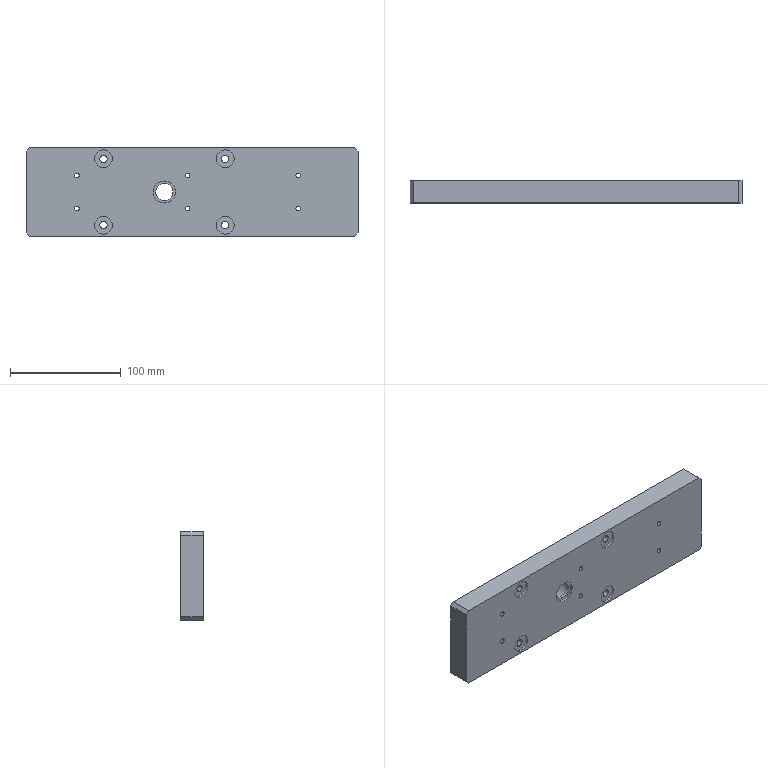Part | SolidWorks | features HoleWzd 4, Chamfer 1, Extrusion 1, ICE 1 | 1 solid | 70 faces | box 300 x 20 x 80 mm | volume 463875 mm3 | cylinder 46 | plane 20 | cone 4 | commonest cylinder face diameters 4.2 x16 6.6 x8 11 x8 16.2 x8 15.5 x2 20 x2